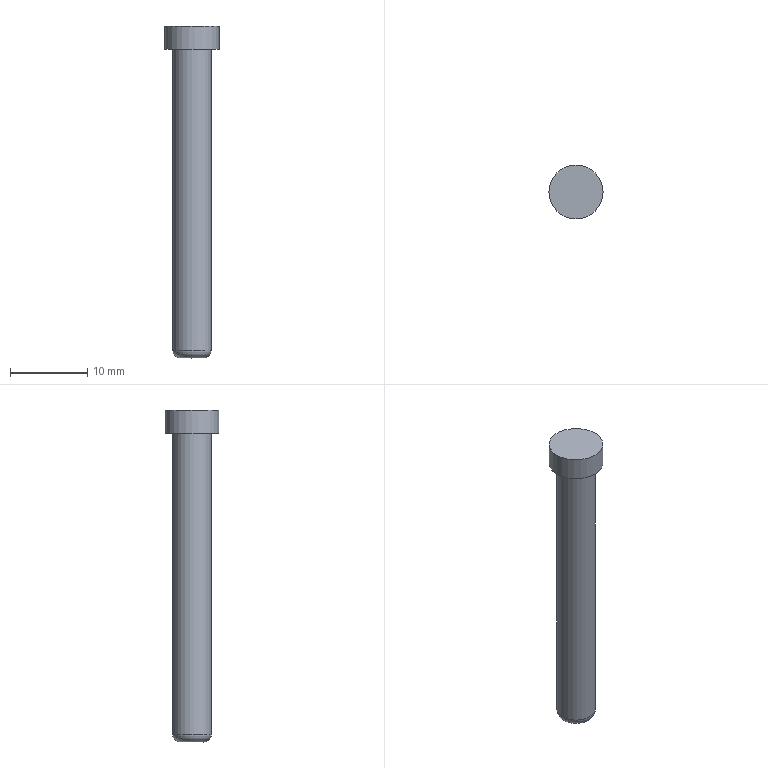Part | NX | features solid 2 | 1 solid | 6 faces | box 7 x 7 x 43 mm | volume 897.781 mm3 | plane 3 | cylinder 2 | torus 1 | commonest cylinder face diameters 5 x1 7 x1
STEP:
#1=CARTESIAN_POINT('',(-190.023,-37.223,47.998));
#2=VERTEX_POINT('',#1);
#3=CARTESIAN_POINT('',(-190.023,-39.723,47.998));
#4=DIRECTION('',(-0.000001665,0.00001617,-1.));
#5=DIRECTION('',(0.,1.,0.00001617));
#6=AXIS2_PLACEMENT_3D('',#3,#4,#5);
#7=CIRCLE('',#6,2.5);
#8=EDGE_CURVE('',#2,#2,#7,.F.);
#9=ORIENTED_EDGE('',*,*,#8,.F.);
#10=EDGE_LOOP('',(#9));
#11=FACE_BOUND('',#10,.T.);
#12=CARTESIAN_POINT('',(-190.023,-37.222,8.998));
#13=VERTEX_POINT('',#12);
#14=CARTESIAN_POINT('',(-190.023,-39.722,8.998));
#15=DIRECTION('',(-0.000001665,0.00001617,-1.));
#16=DIRECTION('',(0.,1.,0.00001617));
#17=AXIS2_PLACEMENT_3D('',#14,#15,#16);
#18=CIRCLE('',#17,2.5);
#19=EDGE_CURVE('',#13,#13,#18,.F.);
#20=ORIENTED_EDGE('',*,*,#19,.T.);
#21=EDGE_LOOP('',(#20));
#22=FACE_BOUND('',#21,.T.);
#23=CARTESIAN_POINT('',(-190.023,-39.723,48.998));
#24=DIRECTION('',(-0.000001665,0.00001617,-1.));
#25=DIRECTION('',(0.,-1.,-0.00001617));
#26=AXIS2_PLACEMENT_3D('',#23,#24,#25);
#27=CYLINDRICAL_SURFACE('',#26,2.5);
#28=ADVANCED_FACE('',(#11,#22),#27,.T.);
#29=CARTESIAN_POINT('',(-190.023,-38.223,7.998));
#30=VERTEX_POINT('',#29);
#31=CARTESIAN_POINT('',(-190.023,-39.722,7.998));
#32=DIRECTION('',(-0.000001665,0.00001617,-1.));
#33=DIRECTION('',(0.,1.,0.00001617));
#34=AXIS2_PLACEMENT_3D('',#31,#32,#33);
#35=CIRCLE('',#34,1.5);
#36=EDGE_CURVE('',#30,#30,#35,.T.);
#37=ORIENTED_EDGE('',*,*,#36,.T.);
#38=EDGE_LOOP('',(#37));
#39=FACE_BOUND('',#38,.T.);
#40=CARTESIAN_POINT('',(-190.023,-39.722,7.998));
#41=DIRECTION('',(-0.000001665,0.00001617,-1.));
#42=DIRECTION('',(0.,-1.,-0.00001617));
#43=AXIS2_PLACEMENT_3D('',#40,#41,#42);
#44=PLANE('',#43);
#45=ADVANCED_FACE('',(#39),#44,.T.);
#46=ORIENTED_EDGE('',*,*,#19,.F.);
#47=EDGE_LOOP('',(#46));
#48=FACE_BOUND('',#47,.T.);
#49=ORIENTED_EDGE('',*,*,#36,.F.);
#50=EDGE_LOOP('',(#49));
#51=FACE_BOUND('',#50,.T.);
#52=CARTESIAN_POINT('',(-190.023,-39.722,8.998));
#53=DIRECTION('',(-0.000001665,0.00001617,-1.));
#54=DIRECTION('',(0.,1.,0.00001617));
#55=AXIS2_PLACEMENT_3D('',#52,#53,#54);
#56=TOROIDAL_SURFACE('',#55,1.5,1.);
#57=ADVANCED_FACE('',(#48,#51),#56,.T.);
#58=CARTESIAN_POINT('',(-186.523,-39.723,50.998));
#59=VERTEX_POINT('',#58);
#60=CARTESIAN_POINT('',(-190.023,-39.723,50.998));
#61=DIRECTION('',(-0.000001665,0.00001617,-1.));
#62=DIRECTION('',(1.,0.,-0.000001665));
#63=AXIS2_PLACEMENT_3D('',#60,#61,#62);
#64=CIRCLE('',#63,3.5);
#65=EDGE_CURVE('',#59,#59,#64,.T.);
#66=ORIENTED_EDGE('',*,*,#65,.T.);
#67=EDGE_LOOP('',(#66));
#68=FACE_BOUND('',#67,.T.);
#69=CARTESIAN_POINT('',(-186.523,-39.723,47.998));
#70=VERTEX_POINT('',#69);
#71=CARTESIAN_POINT('',(-190.023,-39.723,47.998));
#72=DIRECTION('',(-0.000001665,0.00001617,-1.));
#73=DIRECTION('',(1.,0.,-0.000001665));
#74=AXIS2_PLACEMENT_3D('',#71,#72,#73);
#75=CIRCLE('',#74,3.5);
#76=EDGE_CURVE('',#70,#70,#75,.T.);
#77=ORIENTED_EDGE('',*,*,#76,.F.);
#78=EDGE_LOOP('',(#77));
#79=FACE_BOUND('',#78,.T.);
#80=CARTESIAN_POINT('',(-190.023,-39.723,50.998));
#81=DIRECTION('',(-0.000001665,0.00001617,-1.));
#82=DIRECTION('',(0.,-1.,-0.00001617));
#83=AXIS2_PLACEMENT_3D('',#80,#81,#82);
#84=CYLINDRICAL_SURFACE('',#83,3.5);
#85=ADVANCED_FACE('',(#68,#79),#84,.T.);
#86=ORIENTED_EDGE('',*,*,#65,.F.);
#87=EDGE_LOOP('',(#86));
#88=FACE_BOUND('',#87,.T.);
#89=CARTESIAN_POINT('',(-190.023,-39.723,50.998));
#90=DIRECTION('',(-0.000001665,0.00001617,-1.));
#91=DIRECTION('',(0.,-1.,-0.00001617));
#92=AXIS2_PLACEMENT_3D('',#89,#90,#91);
#93=PLANE('',#92);
#94=ADVANCED_FACE('',(#88),#93,.F.);
#95=ORIENTED_EDGE('',*,*,#8,.T.);
#96=EDGE_LOOP('',(#95));
#97=FACE_BOUND('',#96,.T.);
#98=ORIENTED_EDGE('',*,*,#76,.T.);
#99=EDGE_LOOP('',(#98));
#100=FACE_BOUND('',#99,.T.);
#101=CARTESIAN_POINT('',(-190.023,-39.723,47.998));
#102=DIRECTION('',(-0.000001665,0.00001617,-1.));
#103=DIRECTION('',(0.,-1.,-0.00001617));
#104=AXIS2_PLACEMENT_3D('',#101,#102,#103);
#105=PLANE('',#104);
#106=ADVANCED_FACE('',(#97,#100),#105,.T.);
#107=CLOSED_SHELL('',(#28,#45,#57,#85,#94,#106));
#108=MANIFOLD_SOLID_BREP('',#107);
#109=(LENGTH_UNIT()NAMED_UNIT(*)SI_UNIT(.MILLI.,.METRE.));
#110=UNCERTAINTY_MEASURE_WITH_UNIT(LENGTH_MEASURE(0.00001),#109,'','');
#111=(NAMED_UNIT(*)PLANE_ANGLE_UNIT()SI_UNIT($,.RADIAN.));
#112=(NAMED_UNIT(*)SI_UNIT($,.STERADIAN.)SOLID_ANGLE_UNIT());
#113=(GEOMETRIC_REPRESENTATION_CONTEXT(3)GLOBAL_UNCERTAINTY_ASSIGNED_CONTEXT((#110))GLOBAL_UNIT_ASSIGNED_CONTEXT((#109,#111,#112))REPRESENTATION_CONTEXT('',''));
#114=ADVANCED_BREP_SHAPE_REPRESENTATION('',(#108),#113);